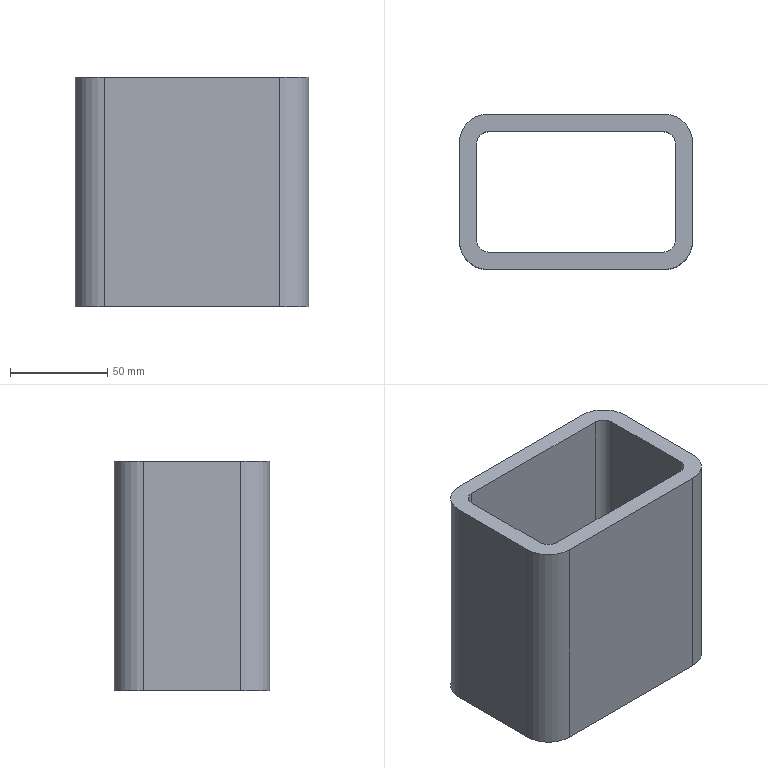Part | SolidWorks | features Fillet 2, Extrusion 1 | 1 solid | 18 faces | box 120 x 80 x 118 mm | volume 367424 mm3 | plane 10 | cylinder 8 | commonest cylinder face diameters 12 x4 30 x4
STEP:
#1=CARTESIAN_POINT('',(-60.,25.,118.));
#2=VERTEX_POINT('',#1);
#3=CARTESIAN_POINT('',(-60.,-25.,118.));
#4=VERTEX_POINT('',#3);
#5=CARTESIAN_POINT('',(-60.,-40.,118.));
#6=DIRECTION('',(0.,-1.,0.));
#7=VECTOR('',#6,1000.);
#8=LINE('',#5,#7);
#9=EDGE_CURVE('',#2,#4,#8,.T.);
#10=ORIENTED_EDGE('',*,*,#9,.T.);
#11=CARTESIAN_POINT('',(-45.,-40.,118.));
#12=VERTEX_POINT('',#11);
#13=CARTESIAN_POINT('',(-45.,-25.,118.));
#14=DIRECTION('',(0.,0.,1.));
#15=DIRECTION('',(-1.,0.,0.));
#16=AXIS2_PLACEMENT_3D('',#13,#14,#15);
#17=CIRCLE('',#16,15.);
#18=EDGE_CURVE('',#4,#12,#17,.T.);
#19=ORIENTED_EDGE('',*,*,#18,.T.);
#20=CARTESIAN_POINT('',(45.,-40.,118.));
#21=VERTEX_POINT('',#20);
#22=CARTESIAN_POINT('',(60.,-40.,118.));
#23=DIRECTION('',(1.,0.,0.));
#24=VECTOR('',#23,1000.);
#25=LINE('',#22,#24);
#26=EDGE_CURVE('',#12,#21,#25,.T.);
#27=ORIENTED_EDGE('',*,*,#26,.T.);
#28=CARTESIAN_POINT('',(60.,-25.,118.));
#29=VERTEX_POINT('',#28);
#30=CARTESIAN_POINT('',(45.,-25.,118.));
#31=DIRECTION('',(0.,0.,1.));
#32=DIRECTION('',(-1.,0.,0.));
#33=AXIS2_PLACEMENT_3D('',#30,#31,#32);
#34=CIRCLE('',#33,15.);
#35=EDGE_CURVE('',#21,#29,#34,.T.);
#36=ORIENTED_EDGE('',*,*,#35,.T.);
#37=CARTESIAN_POINT('',(60.,25.,118.));
#38=VERTEX_POINT('',#37);
#39=CARTESIAN_POINT('',(60.,40.,118.));
#40=DIRECTION('',(0.,1.,0.));
#41=VECTOR('',#40,1000.);
#42=LINE('',#39,#41);
#43=EDGE_CURVE('',#29,#38,#42,.T.);
#44=ORIENTED_EDGE('',*,*,#43,.T.);
#45=CARTESIAN_POINT('',(45.,40.,118.));
#46=VERTEX_POINT('',#45);
#47=CARTESIAN_POINT('',(45.,25.,118.));
#48=DIRECTION('',(0.,0.,1.));
#49=DIRECTION('',(-1.,0.,0.));
#50=AXIS2_PLACEMENT_3D('',#47,#48,#49);
#51=CIRCLE('',#50,15.);
#52=EDGE_CURVE('',#38,#46,#51,.T.);
#53=ORIENTED_EDGE('',*,*,#52,.T.);
#54=CARTESIAN_POINT('',(-45.,40.,118.));
#55=VERTEX_POINT('',#54);
#56=CARTESIAN_POINT('',(-60.,40.,118.));
#57=DIRECTION('',(-1.,0.,0.));
#58=VECTOR('',#57,1000.);
#59=LINE('',#56,#58);
#60=EDGE_CURVE('',#46,#55,#59,.T.);
#61=ORIENTED_EDGE('',*,*,#60,.T.);
#62=CARTESIAN_POINT('',(-45.,25.,118.));
#63=DIRECTION('',(0.,0.,1.));
#64=DIRECTION('',(-1.,0.,0.));
#65=AXIS2_PLACEMENT_3D('',#62,#63,#64);
#66=CIRCLE('',#65,15.);
#67=EDGE_CURVE('',#55,#2,#66,.T.);
#68=ORIENTED_EDGE('',*,*,#67,.T.);
#69=EDGE_LOOP('',(#10,#19,#27,#36,#44,#53,#61,#68));
#70=FACE_OUTER_BOUND('',#69,.T.);
#71=CARTESIAN_POINT('',(-51.,25.,118.));
#72=VERTEX_POINT('',#71);
#73=CARTESIAN_POINT('',(-51.,-25.,118.));
#74=VERTEX_POINT('',#73);
#75=CARTESIAN_POINT('',(-51.,-31.,118.));
#76=DIRECTION('',(0.,-1.,0.));
#77=VECTOR('',#76,1000.);
#78=LINE('',#75,#77);
#79=EDGE_CURVE('',#72,#74,#78,.T.);
#80=ORIENTED_EDGE('',*,*,#79,.F.);
#81=CARTESIAN_POINT('',(-45.,31.,118.));
#82=VERTEX_POINT('',#81);
#83=CARTESIAN_POINT('',(-45.,25.,118.));
#84=DIRECTION('',(0.,0.,-1.));
#85=DIRECTION('',(-1.,0.,0.));
#86=AXIS2_PLACEMENT_3D('',#83,#84,#85);
#87=CIRCLE('',#86,6.);
#88=EDGE_CURVE('',#72,#82,#87,.T.);
#89=ORIENTED_EDGE('',*,*,#88,.T.);
#90=CARTESIAN_POINT('',(45.,31.,118.));
#91=VERTEX_POINT('',#90);
#92=CARTESIAN_POINT('',(-51.,31.,118.));
#93=DIRECTION('',(-1.,0.,0.));
#94=VECTOR('',#93,1000.);
#95=LINE('',#92,#94);
#96=EDGE_CURVE('',#91,#82,#95,.T.);
#97=ORIENTED_EDGE('',*,*,#96,.F.);
#98=CARTESIAN_POINT('',(51.,25.,118.));
#99=VERTEX_POINT('',#98);
#100=CARTESIAN_POINT('',(45.,25.,118.));
#101=DIRECTION('',(0.,0.,-1.));
#102=DIRECTION('',(-1.,0.,0.));
#103=AXIS2_PLACEMENT_3D('',#100,#101,#102);
#104=CIRCLE('',#103,6.);
#105=EDGE_CURVE('',#91,#99,#104,.T.);
#106=ORIENTED_EDGE('',*,*,#105,.T.);
#107=CARTESIAN_POINT('',(51.,-25.,118.));
#108=VERTEX_POINT('',#107);
#109=CARTESIAN_POINT('',(51.,31.,118.));
#110=DIRECTION('',(0.,1.,0.));
#111=VECTOR('',#110,1000.);
#112=LINE('',#109,#111);
#113=EDGE_CURVE('',#108,#99,#112,.T.);
#114=ORIENTED_EDGE('',*,*,#113,.F.);
#115=CARTESIAN_POINT('',(45.,-31.,118.));
#116=VERTEX_POINT('',#115);
#117=CARTESIAN_POINT('',(45.,-25.,118.));
#118=DIRECTION('',(0.,0.,-1.));
#119=DIRECTION('',(-1.,0.,0.));
#120=AXIS2_PLACEMENT_3D('',#117,#118,#119);
#121=CIRCLE('',#120,6.);
#122=EDGE_CURVE('',#108,#116,#121,.T.);
#123=ORIENTED_EDGE('',*,*,#122,.T.);
#124=CARTESIAN_POINT('',(-45.,-31.,118.));
#125=VERTEX_POINT('',#124);
#126=CARTESIAN_POINT('',(51.,-31.,118.));
#127=DIRECTION('',(1.,0.,0.));
#128=VECTOR('',#127,1000.);
#129=LINE('',#126,#128);
#130=EDGE_CURVE('',#125,#116,#129,.T.);
#131=ORIENTED_EDGE('',*,*,#130,.F.);
#132=CARTESIAN_POINT('',(-45.,-25.,118.));
#133=DIRECTION('',(0.,0.,-1.));
#134=DIRECTION('',(-1.,0.,0.));
#135=AXIS2_PLACEMENT_3D('',#132,#133,#134);
#136=CIRCLE('',#135,6.);
#137=EDGE_CURVE('',#125,#74,#136,.T.);
#138=ORIENTED_EDGE('',*,*,#137,.T.);
#139=EDGE_LOOP('',(#80,#89,#97,#106,#114,#123,#131,#138));
#140=FACE_BOUND('',#139,.T.);
#141=CARTESIAN_POINT('',(0.,0.,118.));
#142=DIRECTION('',(0.,0.,-1.));
#143=DIRECTION('',(-1.,0.,0.));
#144=AXIS2_PLACEMENT_3D('',#141,#142,#143);
#145=PLANE('',#144);
#146=ADVANCED_FACE('',(#70,#140),#145,.F.);
#147=CARTESIAN_POINT('',(-45.,-40.,0.));
#148=VERTEX_POINT('',#147);
#149=CARTESIAN_POINT('',(45.,-40.,0.));
#150=VERTEX_POINT('',#149);
#151=CARTESIAN_POINT('',(60.,-40.,0.));
#152=DIRECTION('',(1.,0.,0.));
#153=VECTOR('',#152,1000.);
#154=LINE('',#151,#153);
#155=EDGE_CURVE('',#148,#150,#154,.T.);
#156=ORIENTED_EDGE('',*,*,#155,.F.);
#157=CARTESIAN_POINT('',(-60.,-25.,0.));
#158=VERTEX_POINT('',#157);
#159=CARTESIAN_POINT('',(-45.,-25.,0.));
#160=DIRECTION('',(0.,0.,-1.));
#161=DIRECTION('',(-1.,0.,0.));
#162=AXIS2_PLACEMENT_3D('',#159,#160,#161);
#163=CIRCLE('',#162,15.);
#164=EDGE_CURVE('',#148,#158,#163,.T.);
#165=ORIENTED_EDGE('',*,*,#164,.T.);
#166=CARTESIAN_POINT('',(-60.,25.,0.));
#167=VERTEX_POINT('',#166);
#168=CARTESIAN_POINT('',(-60.,-40.,0.));
#169=DIRECTION('',(0.,-1.,0.));
#170=VECTOR('',#169,1000.);
#171=LINE('',#168,#170);
#172=EDGE_CURVE('',#167,#158,#171,.T.);
#173=ORIENTED_EDGE('',*,*,#172,.F.);
#174=CARTESIAN_POINT('',(-45.,40.,0.));
#175=VERTEX_POINT('',#174);
#176=CARTESIAN_POINT('',(-45.,25.,0.));
#177=DIRECTION('',(0.,0.,-1.));
#178=DIRECTION('',(-1.,0.,0.));
#179=AXIS2_PLACEMENT_3D('',#176,#177,#178);
#180=CIRCLE('',#179,15.);
#181=EDGE_CURVE('',#167,#175,#180,.T.);
#182=ORIENTED_EDGE('',*,*,#181,.T.);
#183=CARTESIAN_POINT('',(45.,40.,0.));
#184=VERTEX_POINT('',#183);
#185=CARTESIAN_POINT('',(-60.,40.,0.));
#186=DIRECTION('',(-1.,0.,0.));
#187=VECTOR('',#186,1000.);
#188=LINE('',#185,#187);
#189=EDGE_CURVE('',#184,#175,#188,.T.);
#190=ORIENTED_EDGE('',*,*,#189,.F.);
#191=CARTESIAN_POINT('',(60.,25.,0.));
#192=VERTEX_POINT('',#191);
#193=CARTESIAN_POINT('',(45.,25.,0.));
#194=DIRECTION('',(0.,0.,-1.));
#195=DIRECTION('',(-1.,0.,0.));
#196=AXIS2_PLACEMENT_3D('',#193,#194,#195);
#197=CIRCLE('',#196,15.);
#198=EDGE_CURVE('',#184,#192,#197,.T.);
#199=ORIENTED_EDGE('',*,*,#198,.T.);
#200=CARTESIAN_POINT('',(60.,-25.,0.));
#201=VERTEX_POINT('',#200);
#202=CARTESIAN_POINT('',(60.,40.,0.));
#203=DIRECTION('',(0.,1.,0.));
#204=VECTOR('',#203,1000.);
#205=LINE('',#202,#204);
#206=EDGE_CURVE('',#201,#192,#205,.T.);
#207=ORIENTED_EDGE('',*,*,#206,.F.);
#208=CARTESIAN_POINT('',(45.,-25.,0.));
#209=DIRECTION('',(0.,0.,-1.));
#210=DIRECTION('',(-1.,0.,0.));
#211=AXIS2_PLACEMENT_3D('',#208,#209,#210);
#212=CIRCLE('',#211,15.);
#213=EDGE_CURVE('',#201,#150,#212,.T.);
#214=ORIENTED_EDGE('',*,*,#213,.T.);
#215=EDGE_LOOP('',(#156,#165,#173,#182,#190,#199,#207,#214));
#216=FACE_OUTER_BOUND('',#215,.T.);
#217=CARTESIAN_POINT('',(51.,-25.,0.));
#218=VERTEX_POINT('',#217);
#219=CARTESIAN_POINT('',(51.,25.,0.));
#220=VERTEX_POINT('',#219);
#221=CARTESIAN_POINT('',(51.,31.,0.));
#222=DIRECTION('',(0.,1.,0.));
#223=VECTOR('',#222,1000.);
#224=LINE('',#221,#223);
#225=EDGE_CURVE('',#218,#220,#224,.T.);
#226=ORIENTED_EDGE('',*,*,#225,.T.);
#227=CARTESIAN_POINT('',(45.,31.,0.));
#228=VERTEX_POINT('',#227);
#229=CARTESIAN_POINT('',(45.,25.,0.));
#230=DIRECTION('',(0.,0.,1.));
#231=DIRECTION('',(-1.,0.,0.));
#232=AXIS2_PLACEMENT_3D('',#229,#230,#231);
#233=CIRCLE('',#232,6.);
#234=EDGE_CURVE('',#220,#228,#233,.T.);
#235=ORIENTED_EDGE('',*,*,#234,.T.);
#236=CARTESIAN_POINT('',(-45.,31.,0.));
#237=VERTEX_POINT('',#236);
#238=CARTESIAN_POINT('',(-51.,31.,0.));
#239=DIRECTION('',(-1.,0.,0.));
#240=VECTOR('',#239,1000.);
#241=LINE('',#238,#240);
#242=EDGE_CURVE('',#228,#237,#241,.T.);
#243=ORIENTED_EDGE('',*,*,#242,.T.);
#244=CARTESIAN_POINT('',(-51.,25.,0.));
#245=VERTEX_POINT('',#244);
#246=CARTESIAN_POINT('',(-45.,25.,0.));
#247=DIRECTION('',(0.,0.,1.));
#248=DIRECTION('',(-1.,0.,0.));
#249=AXIS2_PLACEMENT_3D('',#246,#247,#248);
#250=CIRCLE('',#249,6.);
#251=EDGE_CURVE('',#237,#245,#250,.T.);
#252=ORIENTED_EDGE('',*,*,#251,.T.);
#253=CARTESIAN_POINT('',(-51.,-25.,0.));
#254=VERTEX_POINT('',#253);
#255=CARTESIAN_POINT('',(-51.,-31.,0.));
#256=DIRECTION('',(0.,-1.,0.));
#257=VECTOR('',#256,1000.);
#258=LINE('',#255,#257);
#259=EDGE_CURVE('',#245,#254,#258,.T.);
#260=ORIENTED_EDGE('',*,*,#259,.T.);
#261=CARTESIAN_POINT('',(-45.,-31.,0.));
#262=VERTEX_POINT('',#261);
#263=CARTESIAN_POINT('',(-45.,-25.,0.));
#264=DIRECTION('',(0.,0.,1.));
#265=DIRECTION('',(-1.,0.,0.));
#266=AXIS2_PLACEMENT_3D('',#263,#264,#265);
#267=CIRCLE('',#266,6.);
#268=EDGE_CURVE('',#254,#262,#267,.T.);
#269=ORIENTED_EDGE('',*,*,#268,.T.);
#270=CARTESIAN_POINT('',(45.,-31.,0.));
#271=VERTEX_POINT('',#270);
#272=CARTESIAN_POINT('',(51.,-31.,0.));
#273=DIRECTION('',(1.,0.,0.));
#274=VECTOR('',#273,1000.);
#275=LINE('',#272,#274);
#276=EDGE_CURVE('',#262,#271,#275,.T.);
#277=ORIENTED_EDGE('',*,*,#276,.T.);
#278=CARTESIAN_POINT('',(45.,-25.,0.));
#279=DIRECTION('',(0.,0.,1.));
#280=DIRECTION('',(-1.,0.,0.));
#281=AXIS2_PLACEMENT_3D('',#278,#279,#280);
#282=CIRCLE('',#281,6.);
#283=EDGE_CURVE('',#271,#218,#282,.T.);
#284=ORIENTED_EDGE('',*,*,#283,.T.);
#285=EDGE_LOOP('',(#226,#235,#243,#252,#260,#269,#277,#284));
#286=FACE_BOUND('',#285,.T.);
#287=CARTESIAN_POINT('',(0.,0.,0.));
#288=DIRECTION('',(0.,0.,-1.));
#289=DIRECTION('',(-1.,0.,0.));
#290=AXIS2_PLACEMENT_3D('',#287,#288,#289);
#291=PLANE('',#290);
#292=ADVANCED_FACE('',(#216,#286),#291,.T.);
#293=ORIENTED_EDGE('',*,*,#172,.T.);
#294=CARTESIAN_POINT('',(-60.,-25.,118.));
#295=DIRECTION('',(0.,0.,1.));
#296=VECTOR('',#295,1000.);
#297=LINE('',#294,#296);
#298=EDGE_CURVE('',#158,#4,#297,.T.);
#299=ORIENTED_EDGE('',*,*,#298,.T.);
#300=ORIENTED_EDGE('',*,*,#9,.F.);
#301=CARTESIAN_POINT('',(-60.,25.,118.));
#302=DIRECTION('',(0.,0.,-1.));
#303=VECTOR('',#302,1000.);
#304=LINE('',#301,#303);
#305=EDGE_CURVE('',#2,#167,#304,.T.);
#306=ORIENTED_EDGE('',*,*,#305,.T.);
#307=EDGE_LOOP('',(#293,#299,#300,#306));
#308=FACE_OUTER_BOUND('',#307,.T.);
#309=CARTESIAN_POINT('',(-60.,-40.,118.));
#310=DIRECTION('',(1.,0.,0.));
#311=DIRECTION('',(0.,0.,-1.));
#312=AXIS2_PLACEMENT_3D('',#309,#310,#311);
#313=PLANE('',#312);
#314=ADVANCED_FACE('',(#308),#313,.F.);
#315=ORIENTED_EDGE('',*,*,#26,.F.);
#316=CARTESIAN_POINT('',(-45.,-40.,118.));
#317=DIRECTION('',(0.,0.,-1.));
#318=VECTOR('',#317,1000.);
#319=LINE('',#316,#318);
#320=EDGE_CURVE('',#12,#148,#319,.T.);
#321=ORIENTED_EDGE('',*,*,#320,.T.);
#322=ORIENTED_EDGE('',*,*,#155,.T.);
#323=CARTESIAN_POINT('',(45.,-40.,118.));
#324=DIRECTION('',(0.,0.,1.));
#325=VECTOR('',#324,1000.);
#326=LINE('',#323,#325);
#327=EDGE_CURVE('',#150,#21,#326,.T.);
#328=ORIENTED_EDGE('',*,*,#327,.T.);
#329=EDGE_LOOP('',(#315,#321,#322,#328));
#330=FACE_OUTER_BOUND('',#329,.T.);
#331=CARTESIAN_POINT('',(60.,-40.,118.));
#332=DIRECTION('',(0.,1.,0.));
#333=DIRECTION('',(-1.,0.,0.));
#334=AXIS2_PLACEMENT_3D('',#331,#332,#333);
#335=PLANE('',#334);
#336=ADVANCED_FACE('',(#330),#335,.F.);
#337=ORIENTED_EDGE('',*,*,#43,.F.);
#338=CARTESIAN_POINT('',(60.,-25.,118.));
#339=DIRECTION('',(0.,0.,-1.));
#340=VECTOR('',#339,1000.);
#341=LINE('',#338,#340);
#342=EDGE_CURVE('',#29,#201,#341,.T.);
#343=ORIENTED_EDGE('',*,*,#342,.T.);
#344=ORIENTED_EDGE('',*,*,#206,.T.);
#345=CARTESIAN_POINT('',(60.,25.,118.));
#346=DIRECTION('',(0.,0.,1.));
#347=VECTOR('',#346,1000.);
#348=LINE('',#345,#347);
#349=EDGE_CURVE('',#192,#38,#348,.T.);
#350=ORIENTED_EDGE('',*,*,#349,.T.);
#351=EDGE_LOOP('',(#337,#343,#344,#350));
#352=FACE_OUTER_BOUND('',#351,.T.);
#353=CARTESIAN_POINT('',(60.,40.,118.));
#354=DIRECTION('',(-1.,0.,0.));
#355=DIRECTION('',(0.,-1.,0.));
#356=AXIS2_PLACEMENT_3D('',#353,#354,#355);
#357=PLANE('',#356);
#358=ADVANCED_FACE('',(#352),#357,.F.);
#359=ORIENTED_EDGE('',*,*,#189,.T.);
#360=CARTESIAN_POINT('',(-45.,40.,118.));
#361=DIRECTION('',(0.,0.,1.));
#362=VECTOR('',#361,1000.);
#363=LINE('',#360,#362);
#364=EDGE_CURVE('',#175,#55,#363,.T.);
#365=ORIENTED_EDGE('',*,*,#364,.T.);
#366=ORIENTED_EDGE('',*,*,#60,.F.);
#367=CARTESIAN_POINT('',(45.,40.,118.));
#368=DIRECTION('',(0.,0.,-1.));
#369=VECTOR('',#368,1000.);
#370=LINE('',#367,#369);
#371=EDGE_CURVE('',#46,#184,#370,.T.);
#372=ORIENTED_EDGE('',*,*,#371,.T.);
#373=EDGE_LOOP('',(#359,#365,#366,#372));
#374=FACE_OUTER_BOUND('',#373,.T.);
#375=CARTESIAN_POINT('',(-60.,40.,118.));
#376=DIRECTION('',(0.,-1.,0.));
#377=DIRECTION('',(1.,0.,0.));
#378=AXIS2_PLACEMENT_3D('',#375,#376,#377);
#379=PLANE('',#378);
#380=ADVANCED_FACE('',(#374),#379,.F.);
#381=ORIENTED_EDGE('',*,*,#79,.T.);
#382=CARTESIAN_POINT('',(-51.,-25.,0.));
#383=DIRECTION('',(0.,0.,-1.));
#384=VECTOR('',#383,1000.);
#385=LINE('',#382,#384);
#386=EDGE_CURVE('',#74,#254,#385,.T.);
#387=ORIENTED_EDGE('',*,*,#386,.T.);
#388=ORIENTED_EDGE('',*,*,#259,.F.);
#389=CARTESIAN_POINT('',(-51.,25.,118.));
#390=DIRECTION('',(0.,0.,1.));
#391=VECTOR('',#390,1000.);
#392=LINE('',#389,#391);
#393=EDGE_CURVE('',#245,#72,#392,.T.);
#394=ORIENTED_EDGE('',*,*,#393,.T.);
#395=EDGE_LOOP('',(#381,#387,#388,#394));
#396=FACE_OUTER_BOUND('',#395,.T.);
#397=CARTESIAN_POINT('',(-51.,-31.,118.));
#398=DIRECTION('',(1.,0.,0.));
#399=DIRECTION('',(0.,0.,-1.));
#400=AXIS2_PLACEMENT_3D('',#397,#398,#399);
#401=PLANE('',#400);
#402=ADVANCED_FACE('',(#396),#401,.T.);
#403=ORIENTED_EDGE('',*,*,#130,.T.);
#404=CARTESIAN_POINT('',(45.,-31.,0.));
#405=DIRECTION('',(0.,0.,-1.));
#406=VECTOR('',#405,1000.);
#407=LINE('',#404,#406);
#408=EDGE_CURVE('',#116,#271,#407,.T.);
#409=ORIENTED_EDGE('',*,*,#408,.T.);
#410=ORIENTED_EDGE('',*,*,#276,.F.);
#411=CARTESIAN_POINT('',(-45.,-31.,118.));
#412=DIRECTION('',(0.,0.,1.));
#413=VECTOR('',#412,1000.);
#414=LINE('',#411,#413);
#415=EDGE_CURVE('',#262,#125,#414,.T.);
#416=ORIENTED_EDGE('',*,*,#415,.T.);
#417=EDGE_LOOP('',(#403,#409,#410,#416));
#418=FACE_OUTER_BOUND('',#417,.T.);
#419=CARTESIAN_POINT('',(51.,-31.,118.));
#420=DIRECTION('',(0.,1.,0.));
#421=DIRECTION('',(-1.,0.,0.));
#422=AXIS2_PLACEMENT_3D('',#419,#420,#421);
#423=PLANE('',#422);
#424=ADVANCED_FACE('',(#418),#423,.T.);
#425=ORIENTED_EDGE('',*,*,#113,.T.);
#426=CARTESIAN_POINT('',(51.,25.,0.));
#427=DIRECTION('',(0.,0.,-1.));
#428=VECTOR('',#427,1000.);
#429=LINE('',#426,#428);
#430=EDGE_CURVE('',#99,#220,#429,.T.);
#431=ORIENTED_EDGE('',*,*,#430,.T.);
#432=ORIENTED_EDGE('',*,*,#225,.F.);
#433=CARTESIAN_POINT('',(51.,-25.,118.));
#434=DIRECTION('',(0.,0.,1.));
#435=VECTOR('',#434,1000.);
#436=LINE('',#433,#435);
#437=EDGE_CURVE('',#218,#108,#436,.T.);
#438=ORIENTED_EDGE('',*,*,#437,.T.);
#439=EDGE_LOOP('',(#425,#431,#432,#438));
#440=FACE_OUTER_BOUND('',#439,.T.);
#441=CARTESIAN_POINT('',(51.,31.,118.));
#442=DIRECTION('',(-1.,0.,0.));
#443=DIRECTION('',(0.,-1.,0.));
#444=AXIS2_PLACEMENT_3D('',#441,#442,#443);
#445=PLANE('',#444);
#446=ADVANCED_FACE('',(#440),#445,.T.);
#447=ORIENTED_EDGE('',*,*,#242,.F.);
#448=CARTESIAN_POINT('',(45.,31.,118.));
#449=DIRECTION('',(0.,0.,1.));
#450=VECTOR('',#449,1000.);
#451=LINE('',#448,#450);
#452=EDGE_CURVE('',#228,#91,#451,.T.);
#453=ORIENTED_EDGE('',*,*,#452,.T.);
#454=ORIENTED_EDGE('',*,*,#96,.T.);
#455=CARTESIAN_POINT('',(-45.,31.,0.));
#456=DIRECTION('',(0.,0.,-1.));
#457=VECTOR('',#456,1000.);
#458=LINE('',#455,#457);
#459=EDGE_CURVE('',#82,#237,#458,.T.);
#460=ORIENTED_EDGE('',*,*,#459,.T.);
#461=EDGE_LOOP('',(#447,#453,#454,#460));
#462=FACE_OUTER_BOUND('',#461,.T.);
#463=CARTESIAN_POINT('',(-51.,31.,118.));
#464=DIRECTION('',(0.,-1.,0.));
#465=DIRECTION('',(1.,0.,0.));
#466=AXIS2_PLACEMENT_3D('',#463,#464,#465);
#467=PLANE('',#466);
#468=ADVANCED_FACE('',(#462),#467,.T.);
#469=ORIENTED_EDGE('',*,*,#18,.F.);
#470=ORIENTED_EDGE('',*,*,#298,.F.);
#471=ORIENTED_EDGE('',*,*,#164,.F.);
#472=ORIENTED_EDGE('',*,*,#320,.F.);
#473=EDGE_LOOP('',(#469,#470,#471,#472));
#474=FACE_OUTER_BOUND('',#473,.T.);
#475=CARTESIAN_POINT('',(-45.,-25.,118.));
#476=DIRECTION('',(0.,0.,-1.));
#477=DIRECTION('',(-1.,0.,0.));
#478=AXIS2_PLACEMENT_3D('',#475,#476,#477);
#479=CYLINDRICAL_SURFACE('',#478,15.);
#480=ADVANCED_FACE('',(#474),#479,.T.);
#481=ORIENTED_EDGE('',*,*,#67,.F.);
#482=ORIENTED_EDGE('',*,*,#364,.F.);
#483=ORIENTED_EDGE('',*,*,#181,.F.);
#484=ORIENTED_EDGE('',*,*,#305,.F.);
#485=EDGE_LOOP('',(#481,#482,#483,#484));
#486=FACE_OUTER_BOUND('',#485,.T.);
#487=CARTESIAN_POINT('',(-45.,25.,118.));
#488=DIRECTION('',(0.,0.,-1.));
#489=DIRECTION('',(-1.,0.,0.));
#490=AXIS2_PLACEMENT_3D('',#487,#488,#489);
#491=CYLINDRICAL_SURFACE('',#490,15.);
#492=ADVANCED_FACE('',(#486),#491,.T.);
#493=ORIENTED_EDGE('',*,*,#35,.F.);
#494=ORIENTED_EDGE('',*,*,#327,.F.);
#495=ORIENTED_EDGE('',*,*,#213,.F.);
#496=ORIENTED_EDGE('',*,*,#342,.F.);
#497=EDGE_LOOP('',(#493,#494,#495,#496));
#498=FACE_OUTER_BOUND('',#497,.T.);
#499=CARTESIAN_POINT('',(45.,-25.,118.));
#500=DIRECTION('',(0.,0.,-1.));
#501=DIRECTION('',(-1.,0.,0.));
#502=AXIS2_PLACEMENT_3D('',#499,#500,#501);
#503=CYLINDRICAL_SURFACE('',#502,15.);
#504=ADVANCED_FACE('',(#498),#503,.T.);
#505=ORIENTED_EDGE('',*,*,#52,.F.);
#506=ORIENTED_EDGE('',*,*,#349,.F.);
#507=ORIENTED_EDGE('',*,*,#198,.F.);
#508=ORIENTED_EDGE('',*,*,#371,.F.);
#509=EDGE_LOOP('',(#505,#506,#507,#508));
#510=FACE_OUTER_BOUND('',#509,.T.);
#511=CARTESIAN_POINT('',(45.,25.,118.));
#512=DIRECTION('',(0.,0.,-1.));
#513=DIRECTION('',(-1.,0.,0.));
#514=AXIS2_PLACEMENT_3D('',#511,#512,#513);
#515=CYLINDRICAL_SURFACE('',#514,15.);
#516=ADVANCED_FACE('',(#510),#515,.T.);
#517=ORIENTED_EDGE('',*,*,#105,.F.);
#518=ORIENTED_EDGE('',*,*,#452,.F.);
#519=ORIENTED_EDGE('',*,*,#234,.F.);
#520=ORIENTED_EDGE('',*,*,#430,.F.);
#521=EDGE_LOOP('',(#517,#518,#519,#520));
#522=FACE_OUTER_BOUND('',#521,.T.);
#523=CARTESIAN_POINT('',(45.,25.,118.));
#524=DIRECTION('',(0.,0.,1.));
#525=DIRECTION('',(1.,0.,0.));
#526=AXIS2_PLACEMENT_3D('',#523,#524,#525);
#527=CYLINDRICAL_SURFACE('',#526,6.);
#528=ADVANCED_FACE('',(#522),#527,.F.);
#529=ORIENTED_EDGE('',*,*,#122,.F.);
#530=ORIENTED_EDGE('',*,*,#437,.F.);
#531=ORIENTED_EDGE('',*,*,#283,.F.);
#532=ORIENTED_EDGE('',*,*,#408,.F.);
#533=EDGE_LOOP('',(#529,#530,#531,#532));
#534=FACE_OUTER_BOUND('',#533,.T.);
#535=CARTESIAN_POINT('',(45.,-25.,118.));
#536=DIRECTION('',(0.,0.,1.));
#537=DIRECTION('',(1.,0.,0.));
#538=AXIS2_PLACEMENT_3D('',#535,#536,#537);
#539=CYLINDRICAL_SURFACE('',#538,6.);
#540=ADVANCED_FACE('',(#534),#539,.F.);
#541=ORIENTED_EDGE('',*,*,#137,.F.);
#542=ORIENTED_EDGE('',*,*,#415,.F.);
#543=ORIENTED_EDGE('',*,*,#268,.F.);
#544=ORIENTED_EDGE('',*,*,#386,.F.);
#545=EDGE_LOOP('',(#541,#542,#543,#544));
#546=FACE_OUTER_BOUND('',#545,.T.);
#547=CARTESIAN_POINT('',(-45.,-25.,118.));
#548=DIRECTION('',(0.,0.,1.));
#549=DIRECTION('',(1.,0.,0.));
#550=AXIS2_PLACEMENT_3D('',#547,#548,#549);
#551=CYLINDRICAL_SURFACE('',#550,6.);
#552=ADVANCED_FACE('',(#546),#551,.F.);
#553=ORIENTED_EDGE('',*,*,#88,.F.);
#554=ORIENTED_EDGE('',*,*,#393,.F.);
#555=ORIENTED_EDGE('',*,*,#251,.F.);
#556=ORIENTED_EDGE('',*,*,#459,.F.);
#557=EDGE_LOOP('',(#553,#554,#555,#556));
#558=FACE_OUTER_BOUND('',#557,.T.);
#559=CARTESIAN_POINT('',(-45.,25.,118.));
#560=DIRECTION('',(0.,0.,1.));
#561=DIRECTION('',(1.,0.,0.));
#562=AXIS2_PLACEMENT_3D('',#559,#560,#561);
#563=CYLINDRICAL_SURFACE('',#562,6.);
#564=ADVANCED_FACE('',(#558),#563,.F.);
#565=CLOSED_SHELL('',(#146,#292,#314,#336,#358,#380,#402,#424,#446,#468,#480,#492,#504,#516,#528,#540,#552,#564));
#566=MANIFOLD_SOLID_BREP('',#565);
#567=CARTESIAN_POINT('',(0.,0.,0.));
#568=DIRECTION('',(0.,0.,1.));
#569=DIRECTION('',(1.,0.,0.));
#570=AXIS2_PLACEMENT_3D('',#567,#568,#569);
#571=(LENGTH_UNIT()NAMED_UNIT(*)SI_UNIT(.MILLI.,.METRE.));
#572=UNCERTAINTY_MEASURE_WITH_UNIT(LENGTH_MEASURE(0.00001),#571,'','');
#573=(NAMED_UNIT(*)PLANE_ANGLE_UNIT()SI_UNIT($,.RADIAN.));
#574=(NAMED_UNIT(*)SI_UNIT($,.STERADIAN.)SOLID_ANGLE_UNIT());
#575=(GEOMETRIC_REPRESENTATION_CONTEXT(3)GLOBAL_UNCERTAINTY_ASSIGNED_CONTEXT((#572))GLOBAL_UNIT_ASSIGNED_CONTEXT((#571,#573,#574))REPRESENTATION_CONTEXT('',''));
#576=ADVANCED_BREP_SHAPE_REPRESENTATION('',(#566,#570),#575);